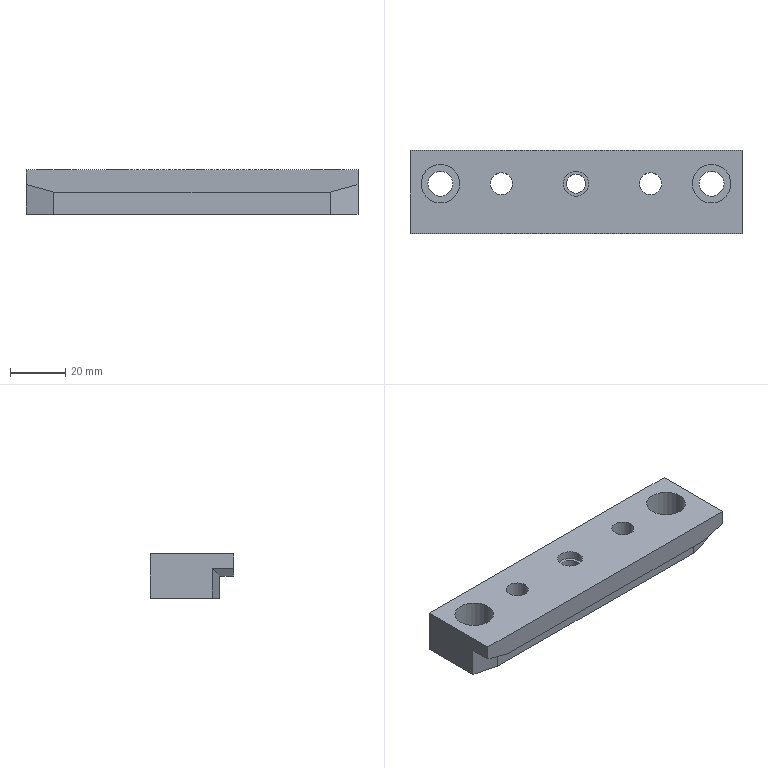Part | STEP file | lll_id4702_x_t | 1 solid | 23 faces | box 120 x 30 x 16 mm | volume 46290 mm3 | plane 15 | cylinder 8 | commonest cylinder face diameters 9 x3 8 x2 14 x2 6.8 x1
STEP:
#1=CARTESIAN_POINT('',(1154.035,355.5,13.));
#2=VERTEX_POINT('',#1);
#3=CARTESIAN_POINT('',(1157.435,355.5,13.));
#4=DIRECTION('',(0.,0.,-1.));
#5=DIRECTION('',(-1.,0.,0.));
#6=AXIS2_PLACEMENT_3D('',#3,#4,#5);
#7=CIRCLE('',#6,3.4);
#8=EDGE_CURVE('',#2,#2,#7,.T.);
#9=ORIENTED_EDGE('',*,*,#8,.T.);
#10=EDGE_LOOP('',(#9));
#11=FACE_BOUND('',#10,.T.);
#12=CARTESIAN_POINT('',(1161.935,355.5,13.));
#13=VERTEX_POINT('',#12);
#14=CARTESIAN_POINT('',(1157.435,355.5,13.));
#15=DIRECTION('',(0.,0.,1.));
#16=DIRECTION('',(1.,0.,0.));
#17=AXIS2_PLACEMENT_3D('',#14,#15,#16);
#18=CIRCLE('',#17,4.5);
#19=EDGE_CURVE('',#13,#13,#18,.T.);
#20=ORIENTED_EDGE('',*,*,#19,.T.);
#21=EDGE_LOOP('',(#20));
#22=FACE_BOUND('',#21,.T.);
#23=CARTESIAN_POINT('',(1157.435,355.5,13.));
#24=DIRECTION('',(0.,0.,-1.));
#25=DIRECTION('',(-1.,0.,0.));
#26=AXIS2_PLACEMENT_3D('',#23,#24,#25);
#27=PLANE('',#26);
#28=ADVANCED_FACE('',(#11,#22),#27,.F.);
#29=CARTESIAN_POINT('',(1201.935,355.5,6.));
#30=VERTEX_POINT('',#29);
#31=CARTESIAN_POINT('',(1206.435,355.5,6.));
#32=DIRECTION('',(0.,0.,-1.));
#33=DIRECTION('',(-1.,0.,0.));
#34=AXIS2_PLACEMENT_3D('',#31,#32,#33);
#35=CIRCLE('',#34,4.5);
#36=EDGE_CURVE('',#30,#30,#35,.T.);
#37=ORIENTED_EDGE('',*,*,#36,.T.);
#38=EDGE_LOOP('',(#37));
#39=FACE_BOUND('',#38,.T.);
#40=CARTESIAN_POINT('',(1213.435,355.5,6.));
#41=VERTEX_POINT('',#40);
#42=CARTESIAN_POINT('',(1206.435,355.5,6.));
#43=DIRECTION('',(0.,0.,1.));
#44=DIRECTION('',(1.,0.,0.));
#45=AXIS2_PLACEMENT_3D('',#42,#43,#44);
#46=CIRCLE('',#45,7.);
#47=EDGE_CURVE('',#41,#41,#46,.T.);
#48=ORIENTED_EDGE('',*,*,#47,.T.);
#49=EDGE_LOOP('',(#48));
#50=FACE_BOUND('',#49,.T.);
#51=CARTESIAN_POINT('',(1206.435,355.5,6.));
#52=DIRECTION('',(0.,0.,-1.));
#53=DIRECTION('',(-1.,0.,0.));
#54=AXIS2_PLACEMENT_3D('',#51,#52,#53);
#55=PLANE('',#54);
#56=ADVANCED_FACE('',(#39,#50),#55,.F.);
#57=CARTESIAN_POINT('',(1207.435,337.5,8.));
#58=VERTEX_POINT('',#57);
#59=CARTESIAN_POINT('',(1217.435,337.5,10.679));
#60=VERTEX_POINT('',#59);
#61=CARTESIAN_POINT('',(1217.435,337.5,10.679));
#62=DIRECTION('',(0.9659,0.,0.2588));
#63=VECTOR('',#62,1.);
#64=LINE('',#61,#63);
#65=EDGE_CURVE('',#58,#60,#64,.T.);
#66=ORIENTED_EDGE('',*,*,#65,.F.);
#67=CARTESIAN_POINT('',(1207.435,342.5,8.));
#68=VERTEX_POINT('',#67);
#69=CARTESIAN_POINT('',(1207.435,324.702,8.));
#70=DIRECTION('',(0.,-1.,0.));
#71=VECTOR('',#70,1.);
#72=LINE('',#69,#71);
#73=EDGE_CURVE('',#68,#58,#72,.T.);
#74=ORIENTED_EDGE('',*,*,#73,.F.);
#75=CARTESIAN_POINT('',(1207.436,342.5,8.));
#76=VERTEX_POINT('',#75);
#77=CARTESIAN_POINT('',(1151.456,342.5,-7.));
#78=DIRECTION('',(-0.9659,0.,-0.2588));
#79=VECTOR('',#78,1.);
#80=LINE('',#77,#79);
#81=EDGE_CURVE('',#76,#68,#80,.T.);
#82=ORIENTED_EDGE('',*,*,#81,.F.);
#83=CARTESIAN_POINT('',(1217.435,345.179,10.679));
#84=VERTEX_POINT('',#83);
#85=CARTESIAN_POINT('',(1207.436,342.5,8.));
#86=DIRECTION('',(-0.9351,-0.2506,-0.2506));
#87=VECTOR('',#86,1.);
#88=LINE('',#85,#87);
#89=EDGE_CURVE('',#84,#76,#88,.T.);
#90=ORIENTED_EDGE('',*,*,#89,.F.);
#91=CARTESIAN_POINT('',(1217.435,337.5,10.679));
#92=DIRECTION('',(0.,1.,0.));
#93=VECTOR('',#92,1.);
#94=LINE('',#91,#93);
#95=EDGE_CURVE('',#60,#84,#94,.T.);
#96=ORIENTED_EDGE('',*,*,#95,.F.);
#97=EDGE_LOOP('',(#66,#74,#82,#90,#96));
#98=FACE_OUTER_BOUND('',#97,.T.);
#99=CARTESIAN_POINT('',(1217.435,337.5,10.679));
#100=DIRECTION('',(-0.2588,0.,0.9659));
#101=DIRECTION('',(0.9659,0.,0.2588));
#102=AXIS2_PLACEMENT_3D('',#99,#100,#101);
#103=PLANE('',#102);
#104=ADVANCED_FACE('',(#98),#103,.F.);
#105=CARTESIAN_POINT('',(1107.435,342.501,8.));
#106=VERTEX_POINT('',#105);
#107=CARTESIAN_POINT('',(1097.435,345.18,10.679));
#108=VERTEX_POINT('',#107);
#109=CARTESIAN_POINT('',(1098.063,345.012,10.511));
#110=DIRECTION('',(-0.9351,0.2506,0.2506));
#111=VECTOR('',#110,1.);
#112=LINE('',#109,#111);
#113=EDGE_CURVE('',#106,#108,#112,.T.);
#114=ORIENTED_EDGE('',*,*,#113,.F.);
#115=CARTESIAN_POINT('',(1107.435,337.5,8.));
#116=VERTEX_POINT('',#115);
#117=CARTESIAN_POINT('',(1107.435,324.702,8.));
#118=DIRECTION('',(0.,1.,0.));
#119=VECTOR('',#118,1.);
#120=LINE('',#117,#119);
#121=EDGE_CURVE('',#116,#106,#120,.T.);
#122=ORIENTED_EDGE('',*,*,#121,.F.);
#123=CARTESIAN_POINT('',(1097.435,337.5,10.679));
#124=VERTEX_POINT('',#123);
#125=CARTESIAN_POINT('',(1097.435,337.5,10.679));
#126=DIRECTION('',(0.9659,0.,-0.2588));
#127=VECTOR('',#126,1.);
#128=LINE('',#125,#127);
#129=EDGE_CURVE('',#124,#116,#128,.T.);
#130=ORIENTED_EDGE('',*,*,#129,.F.);
#131=CARTESIAN_POINT('',(1097.435,367.5,10.679));
#132=DIRECTION('',(0.,-1.,0.));
#133=VECTOR('',#132,1.);
#134=LINE('',#131,#133);
#135=EDGE_CURVE('',#108,#124,#134,.T.);
#136=ORIENTED_EDGE('',*,*,#135,.F.);
#137=EDGE_LOOP('',(#114,#122,#130,#136));
#138=FACE_OUTER_BOUND('',#137,.T.);
#139=CARTESIAN_POINT('',(1097.435,367.5,10.679));
#140=DIRECTION('',(0.2588,0.,0.9659));
#141=DIRECTION('',(0.9659,0.,-0.2588));
#142=AXIS2_PLACEMENT_3D('',#139,#140,#141);
#143=PLANE('',#142);
#144=ADVANCED_FACE('',(#138),#143,.F.);
#145=CARTESIAN_POINT('',(1117.435,337.5,8.));
#146=DIRECTION('',(1.,0.,0.));
#147=VECTOR('',#146,1.);
#148=LINE('',#145,#147);
#149=EDGE_CURVE('',#116,#58,#148,.T.);
#150=ORIENTED_EDGE('',*,*,#149,.F.);
#151=ORIENTED_EDGE('',*,*,#121,.T.);
#152=CARTESIAN_POINT('',(1107.437,342.5,8.));
#153=VERTEX_POINT('',#152);
#154=CARTESIAN_POINT('',(1097.435,345.18,8.));
#155=DIRECTION('',(-0.9659,0.2588,0.));
#156=VECTOR('',#155,1.);
#157=LINE('',#154,#156);
#158=EDGE_CURVE('',#153,#106,#157,.T.);
#159=ORIENTED_EDGE('',*,*,#158,.F.);
#160=CARTESIAN_POINT('',(1127.437,342.5,8.));
#161=DIRECTION('',(-1.,0.,0.));
#162=VECTOR('',#161,1.);
#163=LINE('',#160,#162);
#164=EDGE_CURVE('',#68,#153,#163,.T.);
#165=ORIENTED_EDGE('',*,*,#164,.F.);
#166=ORIENTED_EDGE('',*,*,#73,.T.);
#167=EDGE_LOOP('',(#150,#151,#159,#165,#166));
#168=FACE_OUTER_BOUND('',#167,.T.);
#169=CARTESIAN_POINT('',(1222.025,324.702,8.));
#170=DIRECTION('',(0.,0.,1.));
#171=DIRECTION('',(1.,0.,0.));
#172=AXIS2_PLACEMENT_3D('',#169,#170,#171);
#173=PLANE('',#172);
#174=ADVANCED_FACE('',(#168),#173,.F.);
#175=CARTESIAN_POINT('',(1213.435,355.5,16.));
#176=VERTEX_POINT('',#175);
#177=CARTESIAN_POINT('',(1206.435,355.5,16.));
#178=DIRECTION('',(0.,0.,1.));
#179=DIRECTION('',(1.,0.,0.));
#180=AXIS2_PLACEMENT_3D('',#177,#178,#179);
#181=CIRCLE('',#180,7.);
#182=EDGE_CURVE('',#176,#176,#181,.T.);
#183=ORIENTED_EDGE('',*,*,#182,.T.);
#184=EDGE_LOOP('',(#183));
#185=FACE_BOUND('',#184,.T.);
#186=ORIENTED_EDGE('',*,*,#47,.F.);
#187=EDGE_LOOP('',(#186));
#188=FACE_BOUND('',#187,.T.);
#189=CARTESIAN_POINT('',(1206.435,355.5,47.));
#190=DIRECTION('',(0.,0.,-1.));
#191=DIRECTION('',(-1.,0.,0.));
#192=AXIS2_PLACEMENT_3D('',#189,#190,#191);
#193=CYLINDRICAL_SURFACE('',#192,7.);
#194=ADVANCED_FACE('',(#185,#188),#193,.F.);
#195=CARTESIAN_POINT('',(1097.435,337.5,16.));
#196=VERTEX_POINT('',#195);
#197=CARTESIAN_POINT('',(1097.435,337.5,16.));
#198=DIRECTION('',(0.,0.,-1.));
#199=VECTOR('',#198,1.);
#200=LINE('',#197,#199);
#201=EDGE_CURVE('',#196,#124,#200,.T.);
#202=ORIENTED_EDGE('',*,*,#201,.T.);
#203=ORIENTED_EDGE('',*,*,#129,.T.);
#204=ORIENTED_EDGE('',*,*,#149,.T.);
#205=ORIENTED_EDGE('',*,*,#65,.T.);
#206=CARTESIAN_POINT('',(1217.435,337.5,16.));
#207=VERTEX_POINT('',#206);
#208=CARTESIAN_POINT('',(1217.435,337.5,16.));
#209=DIRECTION('',(0.,0.,-1.));
#210=VECTOR('',#209,1.);
#211=LINE('',#208,#210);
#212=EDGE_CURVE('',#207,#60,#211,.T.);
#213=ORIENTED_EDGE('',*,*,#212,.F.);
#214=CARTESIAN_POINT('',(1117.435,337.5,16.));
#215=DIRECTION('',(1.,0.,0.));
#216=VECTOR('',#215,1.);
#217=LINE('',#214,#216);
#218=EDGE_CURVE('',#196,#207,#217,.T.);
#219=ORIENTED_EDGE('',*,*,#218,.F.);
#220=EDGE_LOOP('',(#202,#203,#204,#205,#213,#219));
#221=FACE_OUTER_BOUND('',#220,.T.);
#222=CARTESIAN_POINT('',(1117.435,337.5,16.));
#223=DIRECTION('',(0.,1.,0.));
#224=DIRECTION('',(0.,0.,1.));
#225=AXIS2_PLACEMENT_3D('',#222,#223,#224);
#226=PLANE('',#225);
#227=ADVANCED_FACE('',(#221),#226,.F.);
#228=ORIENTED_EDGE('',*,*,#8,.F.);
#229=EDGE_LOOP('',(#228));
#230=FACE_BOUND('',#229,.T.);
#231=CARTESIAN_POINT('',(1160.835,355.5,0.));
#232=VERTEX_POINT('',#231);
#233=CARTESIAN_POINT('',(1157.435,355.5,0.));
#234=DIRECTION('',(0.,0.,1.));
#235=DIRECTION('',(1.,0.,0.));
#236=AXIS2_PLACEMENT_3D('',#233,#234,#235);
#237=CIRCLE('',#236,3.4);
#238=EDGE_CURVE('',#232,#232,#237,.T.);
#239=ORIENTED_EDGE('',*,*,#238,.F.);
#240=EDGE_LOOP('',(#239));
#241=FACE_BOUND('',#240,.T.);
#242=CARTESIAN_POINT('',(1157.435,355.5,47.));
#243=DIRECTION('',(0.,0.,-1.));
#244=DIRECTION('',(-1.,0.,0.));
#245=AXIS2_PLACEMENT_3D('',#242,#243,#244);
#246=CYLINDRICAL_SURFACE('',#245,3.4);
#247=ADVANCED_FACE('',(#230,#241),#246,.F.);
#248=ORIENTED_EDGE('',*,*,#36,.F.);
#249=EDGE_LOOP('',(#248));
#250=FACE_BOUND('',#249,.T.);
#251=CARTESIAN_POINT('',(1210.935,355.5,0.));
#252=VERTEX_POINT('',#251);
#253=CARTESIAN_POINT('',(1206.435,355.5,0.));
#254=DIRECTION('',(0.,0.,1.));
#255=DIRECTION('',(1.,0.,0.));
#256=AXIS2_PLACEMENT_3D('',#253,#254,#255);
#257=CIRCLE('',#256,4.5);
#258=EDGE_CURVE('',#252,#252,#257,.T.);
#259=ORIENTED_EDGE('',*,*,#258,.F.);
#260=EDGE_LOOP('',(#259));
#261=FACE_BOUND('',#260,.T.);
#262=CARTESIAN_POINT('',(1206.435,355.5,47.));
#263=DIRECTION('',(0.,0.,-1.));
#264=DIRECTION('',(-1.,0.,0.));
#265=AXIS2_PLACEMENT_3D('',#262,#263,#264);
#266=CYLINDRICAL_SURFACE('',#265,4.5);
#267=ADVANCED_FACE('',(#250,#261),#266,.F.);
#268=CARTESIAN_POINT('',(1107.437,342.5,0.));
#269=VERTEX_POINT('',#268);
#270=CARTESIAN_POINT('',(1207.436,342.5,0.));
#271=VERTEX_POINT('',#270);
#272=CARTESIAN_POINT('',(1127.437,342.5,0.));
#273=DIRECTION('',(1.,0.,0.));
#274=VECTOR('',#273,1.);
#275=LINE('',#272,#274);
#276=EDGE_CURVE('',#269,#271,#275,.T.);
#277=ORIENTED_EDGE('',*,*,#276,.T.);
#278=CARTESIAN_POINT('',(1207.436,342.5,8.));
#279=DIRECTION('',(0.,0.,1.));
#280=VECTOR('',#279,1.);
#281=LINE('',#278,#280);
#282=EDGE_CURVE('',#271,#76,#281,.T.);
#283=ORIENTED_EDGE('',*,*,#282,.T.);
#284=ORIENTED_EDGE('',*,*,#81,.T.);
#285=ORIENTED_EDGE('',*,*,#164,.T.);
#286=CARTESIAN_POINT('',(1107.437,342.5,8.));
#287=DIRECTION('',(0.,0.,1.));
#288=VECTOR('',#287,1.);
#289=LINE('',#286,#288);
#290=EDGE_CURVE('',#269,#153,#289,.T.);
#291=ORIENTED_EDGE('',*,*,#290,.F.);
#292=EDGE_LOOP('',(#277,#283,#284,#285,#291));
#293=FACE_OUTER_BOUND('',#292,.T.);
#294=CARTESIAN_POINT('',(1127.437,342.5,8.));
#295=DIRECTION('',(0.,1.,0.));
#296=DIRECTION('',(0.,0.,1.));
#297=AXIS2_PLACEMENT_3D('',#294,#295,#296);
#298=PLANE('',#297);
#299=ADVANCED_FACE('',(#293),#298,.F.);
#300=CARTESIAN_POINT('',(1217.435,345.179,0.));
#301=VERTEX_POINT('',#300);
#302=CARTESIAN_POINT('',(1207.436,342.5,0.));
#303=DIRECTION('',(0.9659,0.2588,0.));
#304=VECTOR('',#303,1.);
#305=LINE('',#302,#304);
#306=EDGE_CURVE('',#271,#301,#305,.T.);
#307=ORIENTED_EDGE('',*,*,#306,.T.);
#308=CARTESIAN_POINT('',(1217.435,345.179,8.));
#309=DIRECTION('',(0.,0.,-1.));
#310=VECTOR('',#309,1.);
#311=LINE('',#308,#310);
#312=EDGE_CURVE('',#84,#301,#311,.T.);
#313=ORIENTED_EDGE('',*,*,#312,.F.);
#314=ORIENTED_EDGE('',*,*,#89,.T.);
#315=ORIENTED_EDGE('',*,*,#282,.F.);
#316=EDGE_LOOP('',(#307,#313,#314,#315));
#317=FACE_OUTER_BOUND('',#316,.T.);
#318=CARTESIAN_POINT('',(1207.436,342.5,8.));
#319=DIRECTION('',(-0.2588,0.9659,0.));
#320=DIRECTION('',(-0.9659,-0.2588,0.));
#321=AXIS2_PLACEMENT_3D('',#318,#319,#320);
#322=PLANE('',#321);
#323=ADVANCED_FACE('',(#317),#322,.F.);
#324=ORIENTED_EDGE('',*,*,#212,.T.);
#325=ORIENTED_EDGE('',*,*,#95,.T.);
#326=ORIENTED_EDGE('',*,*,#312,.T.);
#327=CARTESIAN_POINT('',(1217.435,367.5,0.));
#328=VERTEX_POINT('',#327);
#329=CARTESIAN_POINT('',(1217.435,337.5,0.));
#330=DIRECTION('',(0.,1.,0.));
#331=VECTOR('',#330,1.);
#332=LINE('',#329,#331);
#333=EDGE_CURVE('',#301,#328,#332,.T.);
#334=ORIENTED_EDGE('',*,*,#333,.T.);
#335=CARTESIAN_POINT('',(1217.435,367.5,16.));
#336=VERTEX_POINT('',#335);
#337=CARTESIAN_POINT('',(1217.435,367.5,16.));
#338=DIRECTION('',(0.,0.,-1.));
#339=VECTOR('',#338,1.);
#340=LINE('',#337,#339);
#341=EDGE_CURVE('',#336,#328,#340,.T.);
#342=ORIENTED_EDGE('',*,*,#341,.F.);
#343=CARTESIAN_POINT('',(1217.435,337.5,16.));
#344=DIRECTION('',(0.,1.,0.));
#345=VECTOR('',#344,1.);
#346=LINE('',#343,#345);
#347=EDGE_CURVE('',#207,#336,#346,.T.);
#348=ORIENTED_EDGE('',*,*,#347,.F.);
#349=EDGE_LOOP('',(#324,#325,#326,#334,#342,#348));
#350=FACE_OUTER_BOUND('',#349,.T.);
#351=CARTESIAN_POINT('',(1217.435,337.5,16.));
#352=DIRECTION('',(-1.,0.,0.));
#353=DIRECTION('',(0.,0.,1.));
#354=AXIS2_PLACEMENT_3D('',#351,#352,#353);
#355=PLANE('',#354);
#356=ADVANCED_FACE('',(#350),#355,.F.);
#357=CARTESIAN_POINT('',(1097.435,367.5,0.));
#358=VERTEX_POINT('',#357);
#359=CARTESIAN_POINT('',(1197.435,367.5,0.));
#360=DIRECTION('',(-1.,0.,0.));
#361=VECTOR('',#360,1.);
#362=LINE('',#359,#361);
#363=EDGE_CURVE('',#328,#358,#362,.T.);
#364=ORIENTED_EDGE('',*,*,#363,.T.);
#365=CARTESIAN_POINT('',(1097.435,367.5,16.));
#366=VERTEX_POINT('',#365);
#367=CARTESIAN_POINT('',(1097.435,367.5,16.));
#368=DIRECTION('',(0.,0.,-1.));
#369=VECTOR('',#368,1.);
#370=LINE('',#367,#369);
#371=EDGE_CURVE('',#366,#358,#370,.T.);
#372=ORIENTED_EDGE('',*,*,#371,.F.);
#373=CARTESIAN_POINT('',(1197.435,367.5,16.));
#374=DIRECTION('',(-1.,0.,0.));
#375=VECTOR('',#374,1.);
#376=LINE('',#373,#375);
#377=EDGE_CURVE('',#336,#366,#376,.T.);
#378=ORIENTED_EDGE('',*,*,#377,.F.);
#379=ORIENTED_EDGE('',*,*,#341,.T.);
#380=EDGE_LOOP('',(#364,#372,#378,#379));
#381=FACE_OUTER_BOUND('',#380,.T.);
#382=CARTESIAN_POINT('',(1197.435,367.5,16.));
#383=DIRECTION('',(0.,-1.,0.));
#384=DIRECTION('',(0.,0.,-1.));
#385=AXIS2_PLACEMENT_3D('',#382,#383,#384);
#386=PLANE('',#385);
#387=ADVANCED_FACE('',(#381),#386,.F.);
#388=CARTESIAN_POINT('',(1097.435,345.18,0.));
#389=VERTEX_POINT('',#388);
#390=CARTESIAN_POINT('',(1097.435,345.18,8.));
#391=DIRECTION('',(0.,0.,-1.));
#392=VECTOR('',#391,1.);
#393=LINE('',#390,#392);
#394=EDGE_CURVE('',#108,#389,#393,.T.);
#395=ORIENTED_EDGE('',*,*,#394,.F.);
#396=ORIENTED_EDGE('',*,*,#135,.T.);
#397=ORIENTED_EDGE('',*,*,#201,.F.);
#398=CARTESIAN_POINT('',(1097.435,367.5,16.));
#399=DIRECTION('',(0.,-1.,0.));
#400=VECTOR('',#399,1.);
#401=LINE('',#398,#400);
#402=EDGE_CURVE('',#366,#196,#401,.T.);
#403=ORIENTED_EDGE('',*,*,#402,.F.);
#404=ORIENTED_EDGE('',*,*,#371,.T.);
#405=CARTESIAN_POINT('',(1097.435,367.5,0.));
#406=DIRECTION('',(0.,-1.,0.));
#407=VECTOR('',#406,1.);
#408=LINE('',#405,#407);
#409=EDGE_CURVE('',#358,#389,#408,.T.);
#410=ORIENTED_EDGE('',*,*,#409,.T.);
#411=EDGE_LOOP('',(#395,#396,#397,#403,#404,#410));
#412=FACE_OUTER_BOUND('',#411,.T.);
#413=CARTESIAN_POINT('',(1097.435,367.5,16.));
#414=DIRECTION('',(1.,0.,0.));
#415=DIRECTION('',(0.,0.,-1.));
#416=AXIS2_PLACEMENT_3D('',#413,#414,#415);
#417=PLANE('',#416);
#418=ADVANCED_FACE('',(#412),#417,.F.);
#419=CARTESIAN_POINT('',(1097.435,345.18,0.));
#420=DIRECTION('',(0.9659,-0.2588,0.));
#421=VECTOR('',#420,1.);
#422=LINE('',#419,#421);
#423=EDGE_CURVE('',#389,#269,#422,.T.);
#424=ORIENTED_EDGE('',*,*,#423,.T.);
#425=ORIENTED_EDGE('',*,*,#290,.T.);
#426=ORIENTED_EDGE('',*,*,#158,.T.);
#427=ORIENTED_EDGE('',*,*,#113,.T.);
#428=ORIENTED_EDGE('',*,*,#394,.T.);
#429=EDGE_LOOP('',(#424,#425,#426,#427,#428));
#430=FACE_OUTER_BOUND('',#429,.T.);
#431=CARTESIAN_POINT('',(1097.435,345.18,8.));
#432=DIRECTION('',(0.2588,0.9659,0.));
#433=DIRECTION('',(-0.9659,0.2588,0.));
#434=AXIS2_PLACEMENT_3D('',#431,#432,#433);
#435=PLANE('',#434);
#436=ADVANCED_FACE('',(#430),#435,.F.);
#437=CARTESIAN_POINT('',(1188.435,355.5,16.));
#438=VERTEX_POINT('',#437);
#439=CARTESIAN_POINT('',(1184.435,355.5,16.));
#440=DIRECTION('',(0.,0.,-1.));
#441=DIRECTION('',(1.,0.,0.));
#442=AXIS2_PLACEMENT_3D('',#439,#440,#441);
#443=CIRCLE('',#442,4.);
#444=EDGE_CURVE('',#438,#438,#443,.T.);
#445=ORIENTED_EDGE('',*,*,#444,.F.);
#446=EDGE_LOOP('',(#445));
#447=FACE_BOUND('',#446,.T.);
#448=CARTESIAN_POINT('',(1188.435,355.5,0.));
#449=VERTEX_POINT('',#448);
#450=CARTESIAN_POINT('',(1184.435,355.5,0.));
#451=DIRECTION('',(0.,0.,1.));
#452=DIRECTION('',(1.,0.,0.));
#453=AXIS2_PLACEMENT_3D('',#450,#451,#452);
#454=CIRCLE('',#453,4.);
#455=EDGE_CURVE('',#449,#449,#454,.T.);
#456=ORIENTED_EDGE('',*,*,#455,.F.);
#457=EDGE_LOOP('',(#456));
#458=FACE_BOUND('',#457,.T.);
#459=CARTESIAN_POINT('',(1184.435,355.5,47.));
#460=DIRECTION('',(0.,0.,-1.));
#461=DIRECTION('',(-1.,0.,0.));
#462=AXIS2_PLACEMENT_3D('',#459,#460,#461);
#463=CYLINDRICAL_SURFACE('',#462,4.);
#464=ADVANCED_FACE('',(#447,#458),#463,.F.);
#465=CARTESIAN_POINT('',(1134.435,355.5,0.));
#466=VERTEX_POINT('',#465);
#467=CARTESIAN_POINT('',(1130.435,355.5,0.));
#468=DIRECTION('',(0.,0.,-1.));
#469=DIRECTION('',(1.,0.,0.));
#470=AXIS2_PLACEMENT_3D('',#467,#468,#469);
#471=CIRCLE('',#470,4.);
#472=EDGE_CURVE('',#466,#466,#471,.T.);
#473=ORIENTED_EDGE('',*,*,#472,.F.);
#474=EDGE_LOOP('',(#473));
#475=FACE_BOUND('',#474,.T.);
#476=ORIENTED_EDGE('',*,*,#455,.T.);
#477=EDGE_LOOP('',(#476));
#478=FACE_BOUND('',#477,.T.);
#479=ORIENTED_EDGE('',*,*,#423,.F.);
#480=ORIENTED_EDGE('',*,*,#409,.F.);
#481=ORIENTED_EDGE('',*,*,#363,.F.);
#482=ORIENTED_EDGE('',*,*,#333,.F.);
#483=ORIENTED_EDGE('',*,*,#306,.F.);
#484=ORIENTED_EDGE('',*,*,#276,.F.);
#485=EDGE_LOOP('',(#479,#480,#481,#482,#483,#484));
#486=FACE_BOUND('',#485,.T.);
#487=ORIENTED_EDGE('',*,*,#258,.T.);
#488=EDGE_LOOP('',(#487));
#489=FACE_BOUND('',#488,.T.);
#490=ORIENTED_EDGE('',*,*,#238,.T.);
#491=EDGE_LOOP('',(#490));
#492=FACE_BOUND('',#491,.T.);
#493=CARTESIAN_POINT('',(1112.935,355.5,0.));
#494=VERTEX_POINT('',#493);
#495=CARTESIAN_POINT('',(1108.435,355.5,0.));
#496=DIRECTION('',(0.,0.,-1.));
#497=DIRECTION('',(1.,0.,0.));
#498=AXIS2_PLACEMENT_3D('',#495,#496,#497);
#499=CIRCLE('',#498,4.5);
#500=EDGE_CURVE('',#494,#494,#499,.T.);
#501=ORIENTED_EDGE('',*,*,#500,.F.);
#502=EDGE_LOOP('',(#501));
#503=FACE_BOUND('',#502,.T.);
#504=CARTESIAN_POINT('',(1117.435,367.5,0.));
#505=DIRECTION('',(0.,0.,1.));
#506=DIRECTION('',(1.,0.,0.));
#507=AXIS2_PLACEMENT_3D('',#504,#505,#506);
#508=PLANE('',#507);
#509=ADVANCED_FACE('',(#475,#478,#486,#489,#492,#503),#508,.F.);
#510=CARTESIAN_POINT('',(1161.935,355.5,16.));
#511=VERTEX_POINT('',#510);
#512=CARTESIAN_POINT('',(1157.435,355.5,16.));
#513=DIRECTION('',(0.,0.,1.));
#514=DIRECTION('',(1.,0.,0.));
#515=AXIS2_PLACEMENT_3D('',#512,#513,#514);
#516=CIRCLE('',#515,4.5);
#517=EDGE_CURVE('',#511,#511,#516,.T.);
#518=ORIENTED_EDGE('',*,*,#517,.T.);
#519=EDGE_LOOP('',(#518));
#520=FACE_BOUND('',#519,.T.);
#521=ORIENTED_EDGE('',*,*,#19,.F.);
#522=EDGE_LOOP('',(#521));
#523=FACE_BOUND('',#522,.T.);
#524=CARTESIAN_POINT('',(1157.435,355.5,47.));
#525=DIRECTION('',(0.,0.,-1.));
#526=DIRECTION('',(-1.,0.,0.));
#527=AXIS2_PLACEMENT_3D('',#524,#525,#526);
#528=CYLINDRICAL_SURFACE('',#527,4.5);
#529=ADVANCED_FACE('',(#520,#523),#528,.F.);
#530=CARTESIAN_POINT('',(1115.435,355.5,16.));
#531=VERTEX_POINT('',#530);
#532=CARTESIAN_POINT('',(1108.435,355.5,16.));
#533=DIRECTION('',(0.,0.,1.));
#534=DIRECTION('',(1.,0.,0.));
#535=AXIS2_PLACEMENT_3D('',#532,#533,#534);
#536=CIRCLE('',#535,7.);
#537=EDGE_CURVE('',#531,#531,#536,.T.);
#538=ORIENTED_EDGE('',*,*,#537,.F.);
#539=EDGE_LOOP('',(#538));
#540=FACE_BOUND('',#539,.T.);
#541=ORIENTED_EDGE('',*,*,#517,.F.);
#542=EDGE_LOOP('',(#541));
#543=FACE_BOUND('',#542,.T.);
#544=ORIENTED_EDGE('',*,*,#377,.T.);
#545=ORIENTED_EDGE('',*,*,#402,.T.);
#546=ORIENTED_EDGE('',*,*,#218,.T.);
#547=ORIENTED_EDGE('',*,*,#347,.T.);
#548=EDGE_LOOP('',(#544,#545,#546,#547));
#549=FACE_BOUND('',#548,.T.);
#550=ORIENTED_EDGE('',*,*,#444,.T.);
#551=EDGE_LOOP('',(#550));
#552=FACE_BOUND('',#551,.T.);
#553=ORIENTED_EDGE('',*,*,#182,.F.);
#554=EDGE_LOOP('',(#553));
#555=FACE_BOUND('',#554,.T.);
#556=CARTESIAN_POINT('',(1134.435,355.5,16.));
#557=VERTEX_POINT('',#556);
#558=CARTESIAN_POINT('',(1130.435,355.5,16.));
#559=DIRECTION('',(0.,0.,-1.));
#560=DIRECTION('',(1.,0.,0.));
#561=AXIS2_PLACEMENT_3D('',#558,#559,#560);
#562=CIRCLE('',#561,4.);
#563=EDGE_CURVE('',#557,#557,#562,.T.);
#564=ORIENTED_EDGE('',*,*,#563,.T.);
#565=EDGE_LOOP('',(#564));
#566=FACE_BOUND('',#565,.T.);
#567=CARTESIAN_POINT('',(1117.435,367.5,16.));
#568=DIRECTION('',(0.,0.,1.));
#569=DIRECTION('',(1.,0.,0.));
#570=AXIS2_PLACEMENT_3D('',#567,#568,#569);
#571=PLANE('',#570);
#572=ADVANCED_FACE('',(#540,#543,#549,#552,#555,#566),#571,.T.);
#573=ORIENTED_EDGE('',*,*,#563,.F.);
#574=EDGE_LOOP('',(#573));
#575=FACE_BOUND('',#574,.T.);
#576=ORIENTED_EDGE('',*,*,#472,.T.);
#577=EDGE_LOOP('',(#576));
#578=FACE_BOUND('',#577,.T.);
#579=CARTESIAN_POINT('',(1130.435,355.5,47.));
#580=DIRECTION('',(0.,0.,-1.));
#581=DIRECTION('',(1.,0.,0.));
#582=AXIS2_PLACEMENT_3D('',#579,#580,#581);
#583=CYLINDRICAL_SURFACE('',#582,4.);
#584=ADVANCED_FACE('',(#575,#578),#583,.F.);
#585=CARTESIAN_POINT('',(1112.935,355.5,6.));
#586=VERTEX_POINT('',#585);
#587=CARTESIAN_POINT('',(1108.435,355.5,6.));
#588=DIRECTION('',(0.,0.,-1.));
#589=DIRECTION('',(1.,0.,0.));
#590=AXIS2_PLACEMENT_3D('',#587,#588,#589);
#591=CIRCLE('',#590,4.5);
#592=EDGE_CURVE('',#586,#586,#591,.T.);
#593=ORIENTED_EDGE('',*,*,#592,.T.);
#594=EDGE_LOOP('',(#593));
#595=FACE_BOUND('',#594,.T.);
#596=CARTESIAN_POINT('',(1101.435,355.5,6.));
#597=VERTEX_POINT('',#596);
#598=CARTESIAN_POINT('',(1108.435,355.5,6.));
#599=DIRECTION('',(0.,0.,1.));
#600=DIRECTION('',(-1.,0.,0.));
#601=AXIS2_PLACEMENT_3D('',#598,#599,#600);
#602=CIRCLE('',#601,7.);
#603=EDGE_CURVE('',#597,#597,#602,.T.);
#604=ORIENTED_EDGE('',*,*,#603,.T.);
#605=EDGE_LOOP('',(#604));
#606=FACE_BOUND('',#605,.T.);
#607=CARTESIAN_POINT('',(1108.435,355.5,6.));
#608=DIRECTION('',(0.,0.,-1.));
#609=DIRECTION('',(1.,0.,0.));
#610=AXIS2_PLACEMENT_3D('',#607,#608,#609);
#611=PLANE('',#610);
#612=ADVANCED_FACE('',(#595,#606),#611,.F.);
#613=ORIENTED_EDGE('',*,*,#592,.F.);
#614=EDGE_LOOP('',(#613));
#615=FACE_BOUND('',#614,.T.);
#616=ORIENTED_EDGE('',*,*,#500,.T.);
#617=EDGE_LOOP('',(#616));
#618=FACE_BOUND('',#617,.T.);
#619=CARTESIAN_POINT('',(1108.435,355.5,47.));
#620=DIRECTION('',(0.,0.,-1.));
#621=DIRECTION('',(1.,0.,0.));
#622=AXIS2_PLACEMENT_3D('',#619,#620,#621);
#623=CYLINDRICAL_SURFACE('',#622,4.5);
#624=ADVANCED_FACE('',(#615,#618),#623,.F.);
#625=ORIENTED_EDGE('',*,*,#537,.T.);
#626=EDGE_LOOP('',(#625));
#627=FACE_BOUND('',#626,.T.);
#628=ORIENTED_EDGE('',*,*,#603,.F.);
#629=EDGE_LOOP('',(#628));
#630=FACE_BOUND('',#629,.T.);
#631=CARTESIAN_POINT('',(1108.435,355.5,47.));
#632=DIRECTION('',(0.,0.,-1.));
#633=DIRECTION('',(1.,0.,0.));
#634=AXIS2_PLACEMENT_3D('',#631,#632,#633);
#635=CYLINDRICAL_SURFACE('',#634,7.);
#636=ADVANCED_FACE('',(#627,#630),#635,.F.);
#637=CLOSED_SHELL('',(#28,#56,#104,#144,#174,#194,#227,#247,#267,#299,#323,#356,#387,#418,#436,#464,#509,#529,#572,#584,#612,#624,#636));
#638=MANIFOLD_SOLID_BREP('',#637);
#639=(LENGTH_UNIT()NAMED_UNIT(*)SI_UNIT(.MILLI.,.METRE.));
#640=UNCERTAINTY_MEASURE_WITH_UNIT(LENGTH_MEASURE(0.00002),#639,'','');
#641=(NAMED_UNIT(*)PLANE_ANGLE_UNIT()SI_UNIT($,.RADIAN.));
#642=PLANE_ANGLE_MEASURE_WITH_UNIT(PLANE_ANGLE_MEASURE(0.01745),#641);
#643=DIMENSIONAL_EXPONENTS(0.,0.,0.,0.,0.,0.,0.);
#644=(CONVERSION_BASED_UNIT('DEGREE',#642)NAMED_UNIT(#643)PLANE_ANGLE_UNIT());
#645=(NAMED_UNIT(*)SI_UNIT($,.STERADIAN.)SOLID_ANGLE_UNIT());
#646=(GEOMETRIC_REPRESENTATION_CONTEXT(3)GLOBAL_UNCERTAINTY_ASSIGNED_CONTEXT((#640))GLOBAL_UNIT_ASSIGNED_CONTEXT((#639,#644,#645))REPRESENTATION_CONTEXT('',''));
#647=ADVANCED_BREP_SHAPE_REPRESENTATION('',(#638),#646);